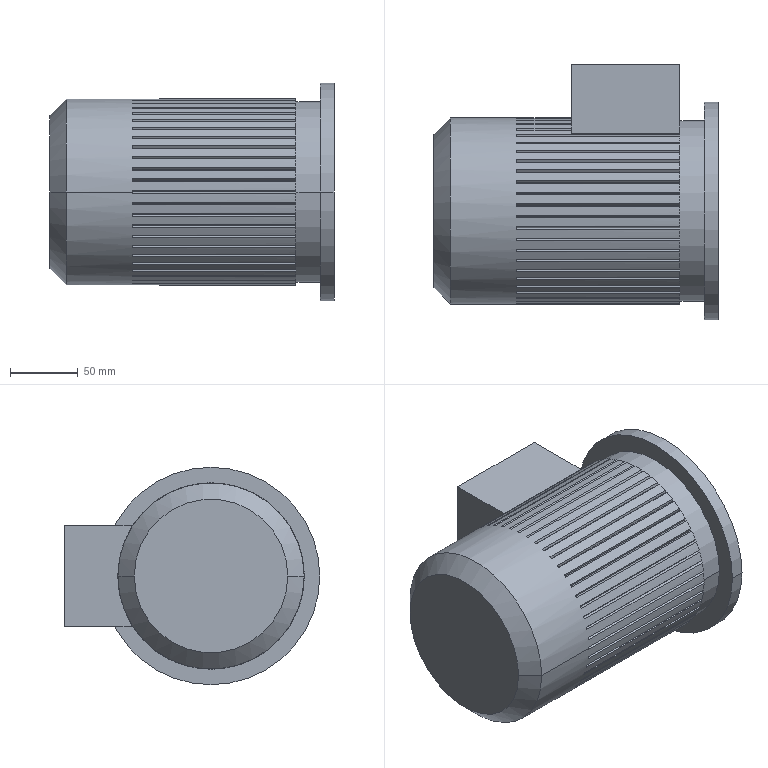Part | 1 solid | 166 faces | box 209 x 188 x 160 mm | volume 3339543 mm3 | plane 158 | cylinder 6 | cone 2 | commonest cylinder face diameters 133 x2 137 x2 160 x2